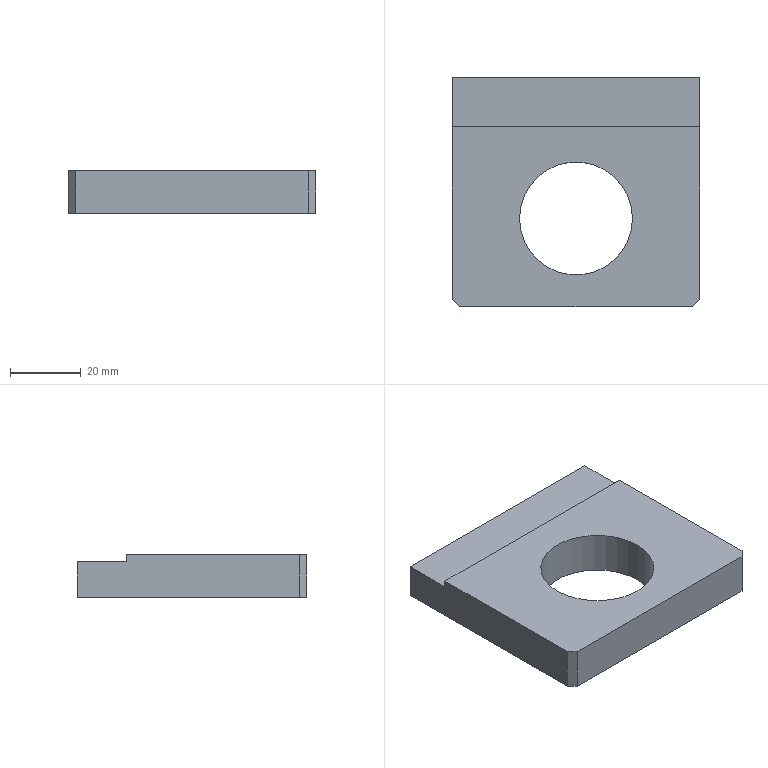Part | STEP file | Backup 2012-3-22-012 | 1 solid | 12 faces | box 70 x 65 x 12 mm | volume 42941 mm3 | plane 10 | cylinder 2 | commonest cylinder face diameters 32 x2
STEP:
#1=CARTESIAN_POINT('',(0.,0.,0.));
#2=DIRECTION('',(0.,0.,1.));
#3=DIRECTION('',(1.,0.,0.));
#4=AXIS2_PLACEMENT_3D('',#1,#2,#3);
#5=CARTESIAN_POINT('',(-16.,-7.5,12.));
#6=VERTEX_POINT('',#5);
#7=CARTESIAN_POINT('',(-16.,-7.5,0.));
#8=VERTEX_POINT('',#7);
#9=CARTESIAN_POINT('',(-16.,-7.5,12.));
#10=DIRECTION('',(0.,0.,-1.));
#11=VECTOR('',#10,1.);
#12=LINE('',#9,#11);
#13=CARTESIAN_POINT('',(0.,-7.5,12.));
#14=DIRECTION('',(0.,0.,-1.));
#15=DIRECTION('',(-1.,0.,0.));
#16=AXIS2_PLACEMENT_3D('',#13,#14,#15);
#17=CYLINDRICAL_SURFACE('',#16,16.);
#18=CARTESIAN_POINT('',(6.283,0.));
#19=DIRECTION('',(0.,1.));
#20=VECTOR('',#19,1.);
#21=LINE('',#18,#20);
#22=(GEOMETRIC_REPRESENTATION_CONTEXT(2)PARAMETRIC_REPRESENTATION_CONTEXT()REPRESENTATION_CONTEXT('',''));
#23=DEFINITIONAL_REPRESENTATION('',(#21),#22);
#24=PCURVE('',#17,#23);
#25=CARTESIAN_POINT('',(0.,-7.5,12.));
#26=DIRECTION('',(0.,0.,-1.));
#27=DIRECTION('',(-1.,0.,0.));
#28=AXIS2_PLACEMENT_3D('',#25,#26,#27);
#29=CYLINDRICAL_SURFACE('',#28,16.);
#30=CARTESIAN_POINT('',(0.,0.));
#31=DIRECTION('',(0.,1.));
#32=VECTOR('',#31,1.);
#33=LINE('',#30,#32);
#34=(GEOMETRIC_REPRESENTATION_CONTEXT(2)PARAMETRIC_REPRESENTATION_CONTEXT()REPRESENTATION_CONTEXT('',''));
#35=DEFINITIONAL_REPRESENTATION('',(#33),#34);
#36=PCURVE('',#29,#35);
#37=SURFACE_CURVE('',#12,(#24,#36),.PCURVE_S1.);
#38=EDGE_CURVE('',#6,#8,#37,.T.);
#39=ORIENTED_EDGE('',*,*,#38,.T.);
#40=CARTESIAN_POINT('',(16.,-7.5,0.));
#41=VERTEX_POINT('',#40);
#42=CARTESIAN_POINT('',(0.,-7.5,0.));
#43=DIRECTION('',(0.,0.,1.));
#44=DIRECTION('',(1.,0.,0.));
#45=AXIS2_PLACEMENT_3D('',#42,#43,#44);
#46=CIRCLE('',#45,16.);
#47=CARTESIAN_POINT('',(9.425,12.));
#48=DIRECTION('',(-1.,0.));
#49=VECTOR('',#48,1.);
#50=LINE('',#47,#49);
#51=(GEOMETRIC_REPRESENTATION_CONTEXT(2)PARAMETRIC_REPRESENTATION_CONTEXT()REPRESENTATION_CONTEXT('',''));
#52=DEFINITIONAL_REPRESENTATION('',(#50),#51);
#53=PCURVE('',#17,#52);
#54=CARTESIAN_POINT('',(35.,-32.5,0.));
#55=DIRECTION('',(0.,0.,1.));
#56=DIRECTION('',(1.,0.,0.));
#57=AXIS2_PLACEMENT_3D('',#54,#55,#56);
#58=PLANE('',#57);
#59=CARTESIAN_POINT('',(-35.,25.));
#60=DIRECTION('',(1.,0.));
#61=AXIS2_PLACEMENT_2D('',#59,#60);
#62=CIRCLE('',#61,16.);
#63=(GEOMETRIC_REPRESENTATION_CONTEXT(2)PARAMETRIC_REPRESENTATION_CONTEXT()REPRESENTATION_CONTEXT('',''));
#64=DEFINITIONAL_REPRESENTATION('',(#62),#63);
#65=PCURVE('',#58,#64);
#66=SURFACE_CURVE('',#46,(#53,#65),.PCURVE_S1.);
#67=EDGE_CURVE('',#8,#41,#66,.T.);
#68=ORIENTED_EDGE('',*,*,#67,.T.);
#69=CARTESIAN_POINT('',(16.,-7.5,12.));
#70=VERTEX_POINT('',#69);
#71=CARTESIAN_POINT('',(16.,-7.5,12.));
#72=DIRECTION('',(0.,0.,-1.));
#73=VECTOR('',#72,1.);
#74=LINE('',#71,#73);
#75=CARTESIAN_POINT('',(3.142,0.));
#76=DIRECTION('',(0.,1.));
#77=VECTOR('',#76,1.);
#78=LINE('',#75,#77);
#79=(GEOMETRIC_REPRESENTATION_CONTEXT(2)PARAMETRIC_REPRESENTATION_CONTEXT()REPRESENTATION_CONTEXT('',''));
#80=DEFINITIONAL_REPRESENTATION('',(#78),#79);
#81=PCURVE('',#17,#80);
#82=CARTESIAN_POINT('',(3.142,0.));
#83=DIRECTION('',(0.,1.));
#84=VECTOR('',#83,1.);
#85=LINE('',#82,#84);
#86=(GEOMETRIC_REPRESENTATION_CONTEXT(2)PARAMETRIC_REPRESENTATION_CONTEXT()REPRESENTATION_CONTEXT('',''));
#87=DEFINITIONAL_REPRESENTATION('',(#85),#86);
#88=PCURVE('',#29,#87);
#89=SURFACE_CURVE('',#74,(#81,#88),.PCURVE_S1.);
#90=EDGE_CURVE('',#70,#41,#89,.T.);
#91=ORIENTED_EDGE('',*,*,#90,.F.);
#92=CARTESIAN_POINT('',(0.,-7.5,12.));
#93=DIRECTION('',(0.,0.,1.));
#94=DIRECTION('',(1.,0.,0.));
#95=AXIS2_PLACEMENT_3D('',#92,#93,#94);
#96=CIRCLE('',#95,16.);
#97=CARTESIAN_POINT('',(9.425,0.));
#98=DIRECTION('',(-1.,0.));
#99=VECTOR('',#98,1.);
#100=LINE('',#97,#99);
#101=(GEOMETRIC_REPRESENTATION_CONTEXT(2)PARAMETRIC_REPRESENTATION_CONTEXT()REPRESENTATION_CONTEXT('',''));
#102=DEFINITIONAL_REPRESENTATION('',(#100),#101);
#103=PCURVE('',#17,#102);
#104=CARTESIAN_POINT('',(35.,-32.5,12.));
#105=DIRECTION('',(0.,0.,1.));
#106=DIRECTION('',(1.,0.,0.));
#107=AXIS2_PLACEMENT_3D('',#104,#105,#106);
#108=PLANE('',#107);
#109=CARTESIAN_POINT('',(-35.,25.));
#110=DIRECTION('',(1.,0.));
#111=AXIS2_PLACEMENT_2D('',#109,#110);
#112=CIRCLE('',#111,16.);
#113=(GEOMETRIC_REPRESENTATION_CONTEXT(2)PARAMETRIC_REPRESENTATION_CONTEXT()REPRESENTATION_CONTEXT('',''));
#114=DEFINITIONAL_REPRESENTATION('',(#112),#113);
#115=PCURVE('',#108,#114);
#116=SURFACE_CURVE('',#96,(#103,#115),.PCURVE_S1.);
#117=EDGE_CURVE('',#6,#70,#116,.T.);
#118=ORIENTED_EDGE('',*,*,#117,.F.);
#119=EDGE_LOOP('',(#39,#68,#91,#118));
#120=FACE_BOUND('',#119,.F.);
#121=ADVANCED_FACE('',(#120),#17,.F.);
#122=CARTESIAN_POINT('',(35.,32.5,10.));
#123=VERTEX_POINT('',#122);
#124=CARTESIAN_POINT('',(-35.,32.5,10.));
#125=VERTEX_POINT('',#124);
#126=CARTESIAN_POINT('',(-35.,32.5,10.));
#127=DIRECTION('',(-1.,0.,0.));
#128=VECTOR('',#127,1.);
#129=LINE('',#126,#128);
#130=CARTESIAN_POINT('',(-35.,32.5,12.));
#131=DIRECTION('',(0.,-1.,0.));
#132=DIRECTION('',(0.,0.,-1.));
#133=AXIS2_PLACEMENT_3D('',#130,#131,#132);
#134=PLANE('',#133);
#135=CARTESIAN_POINT('',(2.,0.));
#136=DIRECTION('',(0.,-1.));
#137=VECTOR('',#136,1.);
#138=LINE('',#135,#137);
#139=(GEOMETRIC_REPRESENTATION_CONTEXT(2)PARAMETRIC_REPRESENTATION_CONTEXT()REPRESENTATION_CONTEXT('',''));
#140=DEFINITIONAL_REPRESENTATION('',(#138),#139);
#141=PCURVE('',#134,#140);
#142=CARTESIAN_POINT('',(-35.,18.5,10.));
#143=DIRECTION('',(0.,0.,1.));
#144=DIRECTION('',(1.,0.,0.));
#145=AXIS2_PLACEMENT_3D('',#142,#143,#144);
#146=PLANE('',#145);
#147=CARTESIAN_POINT('',(0.,14.));
#148=DIRECTION('',(-1.,0.));
#149=VECTOR('',#148,1.);
#150=LINE('',#147,#149);
#151=(GEOMETRIC_REPRESENTATION_CONTEXT(2)PARAMETRIC_REPRESENTATION_CONTEXT()REPRESENTATION_CONTEXT('',''));
#152=DEFINITIONAL_REPRESENTATION('',(#150),#151);
#153=PCURVE('',#146,#152);
#154=SURFACE_CURVE('',#129,(#141,#153),.PCURVE_S1.);
#155=EDGE_CURVE('',#123,#125,#154,.T.);
#156=ORIENTED_EDGE('',*,*,#155,.F.);
#157=CARTESIAN_POINT('',(35.,32.5,0.));
#158=VERTEX_POINT('',#157);
#159=CARTESIAN_POINT('',(35.,32.5,12.));
#160=DIRECTION('',(0.,0.,-1.));
#161=VECTOR('',#160,1.);
#162=LINE('',#159,#161);
#163=CARTESIAN_POINT('',(0.,70.));
#164=DIRECTION('',(1.,0.));
#165=VECTOR('',#164,1.);
#166=LINE('',#163,#165);
#167=(GEOMETRIC_REPRESENTATION_CONTEXT(2)PARAMETRIC_REPRESENTATION_CONTEXT()REPRESENTATION_CONTEXT('',''));
#168=DEFINITIONAL_REPRESENTATION('',(#166),#167);
#169=PCURVE('',#134,#168);
#170=CARTESIAN_POINT('',(35.,32.5,12.));
#171=DIRECTION('',(-1.,0.,0.));
#172=DIRECTION('',(0.,-1.,0.));
#173=AXIS2_PLACEMENT_3D('',#170,#171,#172);
#174=PLANE('',#173);
#175=CARTESIAN_POINT('',(0.,0.));
#176=DIRECTION('',(0.,-1.));
#177=VECTOR('',#176,1.);
#178=LINE('',#175,#177);
#179=(GEOMETRIC_REPRESENTATION_CONTEXT(2)PARAMETRIC_REPRESENTATION_CONTEXT()REPRESENTATION_CONTEXT('',''));
#180=DEFINITIONAL_REPRESENTATION('',(#178),#179);
#181=PCURVE('',#174,#180);
#182=SURFACE_CURVE('',#162,(#169,#181),.PCURVE_S1.);
#183=EDGE_CURVE('',#123,#158,#182,.T.);
#184=ORIENTED_EDGE('',*,*,#183,.T.);
#185=CARTESIAN_POINT('',(-35.,32.5,0.));
#186=VERTEX_POINT('',#185);
#187=CARTESIAN_POINT('',(-35.,32.5,0.));
#188=DIRECTION('',(-1.,0.,0.));
#189=VECTOR('',#188,1.);
#190=LINE('',#187,#189);
#191=CARTESIAN_POINT('',(12.,0.));
#192=DIRECTION('',(0.,-1.));
#193=VECTOR('',#192,1.);
#194=LINE('',#191,#193);
#195=(GEOMETRIC_REPRESENTATION_CONTEXT(2)PARAMETRIC_REPRESENTATION_CONTEXT()REPRESENTATION_CONTEXT('',''));
#196=DEFINITIONAL_REPRESENTATION('',(#194),#195);
#197=PCURVE('',#134,#196);
#198=CARTESIAN_POINT('',(-70.,65.));
#199=DIRECTION('',(-1.,0.));
#200=VECTOR('',#199,1.);
#201=LINE('',#198,#200);
#202=(GEOMETRIC_REPRESENTATION_CONTEXT(2)PARAMETRIC_REPRESENTATION_CONTEXT()REPRESENTATION_CONTEXT('',''));
#203=DEFINITIONAL_REPRESENTATION('',(#201),#202);
#204=PCURVE('',#58,#203);
#205=SURFACE_CURVE('',#190,(#197,#204),.PCURVE_S1.);
#206=EDGE_CURVE('',#158,#186,#205,.T.);
#207=ORIENTED_EDGE('',*,*,#206,.T.);
#208=CARTESIAN_POINT('',(-35.,32.5,12.));
#209=DIRECTION('',(0.,0.,-1.));
#210=VECTOR('',#209,1.);
#211=LINE('',#208,#210);
#212=CARTESIAN_POINT('',(0.,0.));
#213=DIRECTION('',(1.,0.));
#214=VECTOR('',#213,1.);
#215=LINE('',#212,#214);
#216=(GEOMETRIC_REPRESENTATION_CONTEXT(2)PARAMETRIC_REPRESENTATION_CONTEXT()REPRESENTATION_CONTEXT('',''));
#217=DEFINITIONAL_REPRESENTATION('',(#215),#216);
#218=PCURVE('',#134,#217);
#219=CARTESIAN_POINT('',(-35.,32.5,12.));
#220=DIRECTION('',(1.,0.,0.));
#221=DIRECTION('',(0.,1.,0.));
#222=AXIS2_PLACEMENT_3D('',#219,#220,#221);
#223=PLANE('',#222);
#224=CARTESIAN_POINT('',(0.,0.));
#225=DIRECTION('',(0.,-1.));
#226=VECTOR('',#225,1.);
#227=LINE('',#224,#226);
#228=(GEOMETRIC_REPRESENTATION_CONTEXT(2)PARAMETRIC_REPRESENTATION_CONTEXT()REPRESENTATION_CONTEXT('',''));
#229=DEFINITIONAL_REPRESENTATION('',(#227),#228);
#230=PCURVE('',#223,#229);
#231=SURFACE_CURVE('',#211,(#218,#230),.PCURVE_S1.);
#232=EDGE_CURVE('',#125,#186,#231,.T.);
#233=ORIENTED_EDGE('',*,*,#232,.F.);
#234=EDGE_LOOP('',(#156,#184,#207,#233));
#235=FACE_BOUND('',#234,.T.);
#236=ADVANCED_FACE('',(#235),#134,.F.);
#237=CARTESIAN_POINT('',(-33.,-32.5,12.));
#238=VERTEX_POINT('',#237);
#239=CARTESIAN_POINT('',(33.,-32.5,12.));
#240=VERTEX_POINT('',#239);
#241=CARTESIAN_POINT('',(-35.,-32.5,12.));
#242=DIRECTION('',(1.,0.,0.));
#243=VECTOR('',#242,1.);
#244=LINE('',#241,#243);
#245=CARTESIAN_POINT('',(-70.,0.));
#246=DIRECTION('',(1.,0.));
#247=VECTOR('',#246,1.);
#248=LINE('',#245,#247);
#249=(GEOMETRIC_REPRESENTATION_CONTEXT(2)PARAMETRIC_REPRESENTATION_CONTEXT()REPRESENTATION_CONTEXT('',''));
#250=DEFINITIONAL_REPRESENTATION('',(#248),#249);
#251=PCURVE('',#108,#250);
#252=CARTESIAN_POINT('',(-35.,-32.5,12.));
#253=DIRECTION('',(0.,1.,0.));
#254=DIRECTION('',(0.,0.,1.));
#255=AXIS2_PLACEMENT_3D('',#252,#253,#254);
#256=PLANE('',#255);
#257=CARTESIAN_POINT('',(0.,0.));
#258=DIRECTION('',(0.,1.));
#259=VECTOR('',#258,1.);
#260=LINE('',#257,#259);
#261=(GEOMETRIC_REPRESENTATION_CONTEXT(2)PARAMETRIC_REPRESENTATION_CONTEXT()REPRESENTATION_CONTEXT('',''));
#262=DEFINITIONAL_REPRESENTATION('',(#260),#261);
#263=PCURVE('',#256,#262);
#264=SURFACE_CURVE('',#244,(#251,#263),.PCURVE_S1.);
#265=EDGE_CURVE('',#238,#240,#264,.T.);
#266=ORIENTED_EDGE('',*,*,#265,.T.);
#267=CARTESIAN_POINT('',(35.,-30.5,12.));
#268=VERTEX_POINT('',#267);
#269=CARTESIAN_POINT('',(34.,-31.5,12.));
#270=DIRECTION('',(0.7071,0.7071,0.));
#271=VECTOR('',#270,1.);
#272=LINE('',#269,#271);
#273=CARTESIAN_POINT('',(-1.,1.));
#274=DIRECTION('',(0.7071,0.7071));
#275=VECTOR('',#274,1.);
#276=LINE('',#273,#275);
#277=(GEOMETRIC_REPRESENTATION_CONTEXT(2)PARAMETRIC_REPRESENTATION_CONTEXT()REPRESENTATION_CONTEXT('',''));
#278=DEFINITIONAL_REPRESENTATION('',(#276),#277);
#279=PCURVE('',#108,#278);
#280=CARTESIAN_POINT('',(35.,-30.5,12.));
#281=DIRECTION('',(-0.7071,0.7071,0.));
#282=DIRECTION('',(-0.7071,-0.7071,0.));
#283=AXIS2_PLACEMENT_3D('',#280,#281,#282);
#284=PLANE('',#283);
#285=CARTESIAN_POINT('',(1.414,0.));
#286=DIRECTION('',(-1.,0.));
#287=VECTOR('',#286,1.);
#288=LINE('',#285,#287);
#289=(GEOMETRIC_REPRESENTATION_CONTEXT(2)PARAMETRIC_REPRESENTATION_CONTEXT()REPRESENTATION_CONTEXT('',''));
#290=DEFINITIONAL_REPRESENTATION('',(#288),#289);
#291=PCURVE('',#284,#290);
#292=SURFACE_CURVE('',#272,(#279,#291),.PCURVE_S1.);
#293=EDGE_CURVE('',#240,#268,#292,.T.);
#294=ORIENTED_EDGE('',*,*,#293,.T.);
#295=CARTESIAN_POINT('',(35.,18.5,12.));
#296=VERTEX_POINT('',#295);
#297=CARTESIAN_POINT('',(35.,32.5,12.));
#298=DIRECTION('',(0.,1.,0.));
#299=VECTOR('',#298,1.);
#300=LINE('',#297,#299);
#301=CARTESIAN_POINT('',(0.,65.));
#302=DIRECTION('',(0.,1.));
#303=VECTOR('',#302,1.);
#304=LINE('',#301,#303);
#305=(GEOMETRIC_REPRESENTATION_CONTEXT(2)PARAMETRIC_REPRESENTATION_CONTEXT()REPRESENTATION_CONTEXT('',''));
#306=DEFINITIONAL_REPRESENTATION('',(#304),#305);
#307=PCURVE('',#108,#306);
#308=CARTESIAN_POINT('',(0.,0.));
#309=DIRECTION('',(-1.,0.));
#310=VECTOR('',#309,1.);
#311=LINE('',#308,#310);
#312=(GEOMETRIC_REPRESENTATION_CONTEXT(2)PARAMETRIC_REPRESENTATION_CONTEXT()REPRESENTATION_CONTEXT('',''));
#313=DEFINITIONAL_REPRESENTATION('',(#311),#312);
#314=PCURVE('',#174,#313);
#315=SURFACE_CURVE('',#300,(#307,#314),.PCURVE_S1.);
#316=EDGE_CURVE('',#268,#296,#315,.T.);
#317=ORIENTED_EDGE('',*,*,#316,.T.);
#318=CARTESIAN_POINT('',(-35.,18.5,12.));
#319=VERTEX_POINT('',#318);
#320=CARTESIAN_POINT('',(-35.,18.5,12.));
#321=DIRECTION('',(1.,0.,0.));
#322=VECTOR('',#321,1.);
#323=LINE('',#320,#322);
#324=CARTESIAN_POINT('',(-70.,51.));
#325=DIRECTION('',(1.,0.));
#326=VECTOR('',#325,1.);
#327=LINE('',#324,#326);
#328=(GEOMETRIC_REPRESENTATION_CONTEXT(2)PARAMETRIC_REPRESENTATION_CONTEXT()REPRESENTATION_CONTEXT('',''));
#329=DEFINITIONAL_REPRESENTATION('',(#327),#328);
#330=PCURVE('',#108,#329);
#331=CARTESIAN_POINT('',(-35.,18.5,10.));
#332=DIRECTION('',(0.,-1.,0.));
#333=DIRECTION('',(1.,0.,0.));
#334=AXIS2_PLACEMENT_3D('',#331,#332,#333);
#335=PLANE('',#334);
#336=CARTESIAN_POINT('',(0.,2.));
#337=DIRECTION('',(1.,0.));
#338=VECTOR('',#337,1.);
#339=LINE('',#336,#338);
#340=(GEOMETRIC_REPRESENTATION_CONTEXT(2)PARAMETRIC_REPRESENTATION_CONTEXT()REPRESENTATION_CONTEXT('',''));
#341=DEFINITIONAL_REPRESENTATION('',(#339),#340);
#342=PCURVE('',#335,#341);
#343=SURFACE_CURVE('',#323,(#330,#342),.PCURVE_S1.);
#344=EDGE_CURVE('',#319,#296,#343,.T.);
#345=ORIENTED_EDGE('',*,*,#344,.F.);
#346=CARTESIAN_POINT('',(-35.,-30.5,12.));
#347=VERTEX_POINT('',#346);
#348=CARTESIAN_POINT('',(-35.,32.5,12.));
#349=DIRECTION('',(0.,-1.,0.));
#350=VECTOR('',#349,1.);
#351=LINE('',#348,#350);
#352=CARTESIAN_POINT('',(-70.,65.));
#353=DIRECTION('',(0.,-1.));
#354=VECTOR('',#353,1.);
#355=LINE('',#352,#354);
#356=(GEOMETRIC_REPRESENTATION_CONTEXT(2)PARAMETRIC_REPRESENTATION_CONTEXT()REPRESENTATION_CONTEXT('',''));
#357=DEFINITIONAL_REPRESENTATION('',(#355),#356);
#358=PCURVE('',#108,#357);
#359=CARTESIAN_POINT('',(0.,0.));
#360=DIRECTION('',(-1.,0.));
#361=VECTOR('',#360,1.);
#362=LINE('',#359,#361);
#363=(GEOMETRIC_REPRESENTATION_CONTEXT(2)PARAMETRIC_REPRESENTATION_CONTEXT()REPRESENTATION_CONTEXT('',''));
#364=DEFINITIONAL_REPRESENTATION('',(#362),#363);
#365=PCURVE('',#223,#364);
#366=SURFACE_CURVE('',#351,(#358,#365),.PCURVE_S1.);
#367=EDGE_CURVE('',#319,#347,#366,.T.);
#368=ORIENTED_EDGE('',*,*,#367,.T.);
#369=CARTESIAN_POINT('',(1.,-66.5,12.));
#370=DIRECTION('',(0.7071,-0.7071,0.));
#371=VECTOR('',#370,1.);
#372=LINE('',#369,#371);
#373=CARTESIAN_POINT('',(-34.,-34.));
#374=DIRECTION('',(0.7071,-0.7071));
#375=VECTOR('',#374,1.);
#376=LINE('',#373,#375);
#377=(GEOMETRIC_REPRESENTATION_CONTEXT(2)PARAMETRIC_REPRESENTATION_CONTEXT()REPRESENTATION_CONTEXT('',''));
#378=DEFINITIONAL_REPRESENTATION('',(#376),#377);
#379=PCURVE('',#108,#378);
#380=CARTESIAN_POINT('',(-33.,-32.5,12.));
#381=DIRECTION('',(0.7071,0.7071,0.));
#382=DIRECTION('',(-0.7071,0.7071,0.));
#383=AXIS2_PLACEMENT_3D('',#380,#381,#382);
#384=PLANE('',#383);
#385=CARTESIAN_POINT('',(-48.083,0.));
#386=DIRECTION('',(-1.,0.));
#387=VECTOR('',#386,1.);
#388=LINE('',#385,#387);
#389=(GEOMETRIC_REPRESENTATION_CONTEXT(2)PARAMETRIC_REPRESENTATION_CONTEXT()REPRESENTATION_CONTEXT('',''));
#390=DEFINITIONAL_REPRESENTATION('',(#388),#389);
#391=PCURVE('',#384,#390);
#392=SURFACE_CURVE('',#372,(#379,#391),.PCURVE_S1.);
#393=EDGE_CURVE('',#347,#238,#392,.T.);
#394=ORIENTED_EDGE('',*,*,#393,.T.);
#395=EDGE_LOOP('',(#266,#294,#317,#345,#368,#394));
#396=FACE_BOUND('',#395,.T.);
#397=ORIENTED_EDGE('',*,*,#117,.F.);
#398=CARTESIAN_POINT('',(0.,-7.5,12.));
#399=DIRECTION('',(0.,0.,1.));
#400=DIRECTION('',(1.,0.,0.));
#401=AXIS2_PLACEMENT_3D('',#398,#399,#400);
#402=CIRCLE('',#401,16.);
#403=CARTESIAN_POINT('',(-35.,25.));
#404=DIRECTION('',(1.,0.));
#405=AXIS2_PLACEMENT_2D('',#403,#404);
#406=CIRCLE('',#405,16.);
#407=(GEOMETRIC_REPRESENTATION_CONTEXT(2)PARAMETRIC_REPRESENTATION_CONTEXT()REPRESENTATION_CONTEXT('',''));
#408=DEFINITIONAL_REPRESENTATION('',(#406),#407);
#409=PCURVE('',#108,#408);
#410=CARTESIAN_POINT('',(3.142,0.));
#411=DIRECTION('',(-1.,0.));
#412=VECTOR('',#411,1.);
#413=LINE('',#410,#412);
#414=(GEOMETRIC_REPRESENTATION_CONTEXT(2)PARAMETRIC_REPRESENTATION_CONTEXT()REPRESENTATION_CONTEXT('',''));
#415=DEFINITIONAL_REPRESENTATION('',(#413),#414);
#416=PCURVE('',#29,#415);
#417=SURFACE_CURVE('',#402,(#409,#416),.PCURVE_S1.);
#418=EDGE_CURVE('',#70,#6,#417,.T.);
#419=ORIENTED_EDGE('',*,*,#418,.F.);
#420=EDGE_LOOP('',(#397,#419));
#421=FACE_BOUND('',#420,.T.);
#422=ADVANCED_FACE('',(#396,#421),#108,.T.);
#423=CARTESIAN_POINT('',(35.,-30.5,0.));
#424=VERTEX_POINT('',#423);
#425=CARTESIAN_POINT('',(35.,32.5,0.));
#426=DIRECTION('',(0.,1.,0.));
#427=VECTOR('',#426,1.);
#428=LINE('',#425,#427);
#429=CARTESIAN_POINT('',(0.,65.));
#430=DIRECTION('',(0.,1.));
#431=VECTOR('',#430,1.);
#432=LINE('',#429,#431);
#433=(GEOMETRIC_REPRESENTATION_CONTEXT(2)PARAMETRIC_REPRESENTATION_CONTEXT()REPRESENTATION_CONTEXT('',''));
#434=DEFINITIONAL_REPRESENTATION('',(#432),#433);
#435=PCURVE('',#58,#434);
#436=CARTESIAN_POINT('',(0.,-12.));
#437=DIRECTION('',(-1.,0.));
#438=VECTOR('',#437,1.);
#439=LINE('',#436,#438);
#440=(GEOMETRIC_REPRESENTATION_CONTEXT(2)PARAMETRIC_REPRESENTATION_CONTEXT()REPRESENTATION_CONTEXT('',''));
#441=DEFINITIONAL_REPRESENTATION('',(#439),#440);
#442=PCURVE('',#174,#441);
#443=SURFACE_CURVE('',#428,(#435,#442),.PCURVE_S1.);
#444=EDGE_CURVE('',#424,#158,#443,.T.);
#445=ORIENTED_EDGE('',*,*,#444,.F.);
#446=CARTESIAN_POINT('',(33.,-32.5,0.));
#447=VERTEX_POINT('',#446);
#448=CARTESIAN_POINT('',(35.,-30.5,0.));
#449=DIRECTION('',(-0.7071,-0.7071,0.));
#450=VECTOR('',#449,1.);
#451=LINE('',#448,#450);
#452=CARTESIAN_POINT('',(0.,2.));
#453=DIRECTION('',(-0.7071,-0.7071));
#454=VECTOR('',#453,1.);
#455=LINE('',#452,#454);
#456=(GEOMETRIC_REPRESENTATION_CONTEXT(2)PARAMETRIC_REPRESENTATION_CONTEXT()REPRESENTATION_CONTEXT('',''));
#457=DEFINITIONAL_REPRESENTATION('',(#455),#456);
#458=PCURVE('',#58,#457);
#459=CARTESIAN_POINT('',(0.,-12.));
#460=DIRECTION('',(1.,0.));
#461=VECTOR('',#460,1.);
#462=LINE('',#459,#461);
#463=(GEOMETRIC_REPRESENTATION_CONTEXT(2)PARAMETRIC_REPRESENTATION_CONTEXT()REPRESENTATION_CONTEXT('',''));
#464=DEFINITIONAL_REPRESENTATION('',(#462),#463);
#465=PCURVE('',#284,#464);
#466=SURFACE_CURVE('',#451,(#458,#465),.PCURVE_S1.);
#467=EDGE_CURVE('',#424,#447,#466,.T.);
#468=ORIENTED_EDGE('',*,*,#467,.T.);
#469=CARTESIAN_POINT('',(-33.,-32.5,0.));
#470=VERTEX_POINT('',#469);
#471=CARTESIAN_POINT('',(-35.,-32.5,0.));
#472=DIRECTION('',(1.,0.,0.));
#473=VECTOR('',#472,1.);
#474=LINE('',#471,#473);
#475=CARTESIAN_POINT('',(-70.,0.));
#476=DIRECTION('',(1.,0.));
#477=VECTOR('',#476,1.);
#478=LINE('',#475,#477);
#479=(GEOMETRIC_REPRESENTATION_CONTEXT(2)PARAMETRIC_REPRESENTATION_CONTEXT()REPRESENTATION_CONTEXT('',''));
#480=DEFINITIONAL_REPRESENTATION('',(#478),#479);
#481=PCURVE('',#58,#480);
#482=CARTESIAN_POINT('',(-12.,0.));
#483=DIRECTION('',(0.,1.));
#484=VECTOR('',#483,1.);
#485=LINE('',#482,#484);
#486=(GEOMETRIC_REPRESENTATION_CONTEXT(2)PARAMETRIC_REPRESENTATION_CONTEXT()REPRESENTATION_CONTEXT('',''));
#487=DEFINITIONAL_REPRESENTATION('',(#485),#486);
#488=PCURVE('',#256,#487);
#489=SURFACE_CURVE('',#474,(#481,#488),.PCURVE_S1.);
#490=EDGE_CURVE('',#470,#447,#489,.T.);
#491=ORIENTED_EDGE('',*,*,#490,.F.);
#492=CARTESIAN_POINT('',(-35.,-30.5,0.));
#493=VERTEX_POINT('',#492);
#494=CARTESIAN_POINT('',(-33.,-32.5,0.));
#495=DIRECTION('',(-0.7071,0.7071,0.));
#496=VECTOR('',#495,1.);
#497=LINE('',#494,#496);
#498=CARTESIAN_POINT('',(-68.,0.));
#499=DIRECTION('',(-0.7071,0.7071));
#500=VECTOR('',#499,1.);
#501=LINE('',#498,#500);
#502=(GEOMETRIC_REPRESENTATION_CONTEXT(2)PARAMETRIC_REPRESENTATION_CONTEXT()REPRESENTATION_CONTEXT('',''));
#503=DEFINITIONAL_REPRESENTATION('',(#501),#502);
#504=PCURVE('',#58,#503);
#505=CARTESIAN_POINT('',(0.,-12.));
#506=DIRECTION('',(1.,0.));
#507=VECTOR('',#506,1.);
#508=LINE('',#505,#507);
#509=(GEOMETRIC_REPRESENTATION_CONTEXT(2)PARAMETRIC_REPRESENTATION_CONTEXT()REPRESENTATION_CONTEXT('',''));
#510=DEFINITIONAL_REPRESENTATION('',(#508),#509);
#511=PCURVE('',#384,#510);
#512=SURFACE_CURVE('',#497,(#504,#511),.PCURVE_S1.);
#513=EDGE_CURVE('',#470,#493,#512,.T.);
#514=ORIENTED_EDGE('',*,*,#513,.T.);
#515=CARTESIAN_POINT('',(-35.,32.5,0.));
#516=DIRECTION('',(0.,-1.,0.));
#517=VECTOR('',#516,1.);
#518=LINE('',#515,#517);
#519=CARTESIAN_POINT('',(-70.,65.));
#520=DIRECTION('',(0.,-1.));
#521=VECTOR('',#520,1.);
#522=LINE('',#519,#521);
#523=(GEOMETRIC_REPRESENTATION_CONTEXT(2)PARAMETRIC_REPRESENTATION_CONTEXT()REPRESENTATION_CONTEXT('',''));
#524=DEFINITIONAL_REPRESENTATION('',(#522),#523);
#525=PCURVE('',#58,#524);
#526=CARTESIAN_POINT('',(0.,-12.));
#527=DIRECTION('',(-1.,0.));
#528=VECTOR('',#527,1.);
#529=LINE('',#526,#528);
#530=(GEOMETRIC_REPRESENTATION_CONTEXT(2)PARAMETRIC_REPRESENTATION_CONTEXT()REPRESENTATION_CONTEXT('',''));
#531=DEFINITIONAL_REPRESENTATION('',(#529),#530);
#532=PCURVE('',#223,#531);
#533=SURFACE_CURVE('',#518,(#525,#532),.PCURVE_S1.);
#534=EDGE_CURVE('',#186,#493,#533,.T.);
#535=ORIENTED_EDGE('',*,*,#534,.F.);
#536=ORIENTED_EDGE('',*,*,#206,.F.);
#537=EDGE_LOOP('',(#445,#468,#491,#514,#535,#536));
#538=FACE_BOUND('',#537,.T.);
#539=ORIENTED_EDGE('',*,*,#67,.T.);
#540=CARTESIAN_POINT('',(0.,-7.5,0.));
#541=DIRECTION('',(0.,0.,1.));
#542=DIRECTION('',(1.,0.,0.));
#543=AXIS2_PLACEMENT_3D('',#540,#541,#542);
#544=CIRCLE('',#543,16.);
#545=CARTESIAN_POINT('',(-35.,25.));
#546=DIRECTION('',(1.,0.));
#547=AXIS2_PLACEMENT_2D('',#545,#546);
#548=CIRCLE('',#547,16.);
#549=(GEOMETRIC_REPRESENTATION_CONTEXT(2)PARAMETRIC_REPRESENTATION_CONTEXT()REPRESENTATION_CONTEXT('',''));
#550=DEFINITIONAL_REPRESENTATION('',(#548),#549);
#551=PCURVE('',#58,#550);
#552=CARTESIAN_POINT('',(3.142,12.));
#553=DIRECTION('',(-1.,0.));
#554=VECTOR('',#553,1.);
#555=LINE('',#552,#554);
#556=(GEOMETRIC_REPRESENTATION_CONTEXT(2)PARAMETRIC_REPRESENTATION_CONTEXT()REPRESENTATION_CONTEXT('',''));
#557=DEFINITIONAL_REPRESENTATION('',(#555),#556);
#558=PCURVE('',#29,#557);
#559=SURFACE_CURVE('',#544,(#551,#558),.PCURVE_S1.);
#560=EDGE_CURVE('',#41,#8,#559,.T.);
#561=ORIENTED_EDGE('',*,*,#560,.T.);
#562=EDGE_LOOP('',(#539,#561));
#563=FACE_BOUND('',#562,.T.);
#564=ADVANCED_FACE('',(#538,#563),#58,.F.);
#565=ORIENTED_EDGE('',*,*,#316,.F.);
#566=CARTESIAN_POINT('',(35.,-30.5,12.));
#567=DIRECTION('',(0.,0.,-1.));
#568=VECTOR('',#567,1.);
#569=LINE('',#566,#568);
#570=CARTESIAN_POINT('',(63.,0.));
#571=DIRECTION('',(0.,-1.));
#572=VECTOR('',#571,1.);
#573=LINE('',#570,#572);
#574=(GEOMETRIC_REPRESENTATION_CONTEXT(2)PARAMETRIC_REPRESENTATION_CONTEXT()REPRESENTATION_CONTEXT('',''));
#575=DEFINITIONAL_REPRESENTATION('',(#573),#574);
#576=PCURVE('',#174,#575);
#577=CARTESIAN_POINT('',(0.,0.));
#578=DIRECTION('',(0.,-1.));
#579=VECTOR('',#578,1.);
#580=LINE('',#577,#579);
#581=(GEOMETRIC_REPRESENTATION_CONTEXT(2)PARAMETRIC_REPRESENTATION_CONTEXT()REPRESENTATION_CONTEXT('',''));
#582=DEFINITIONAL_REPRESENTATION('',(#580),#581);
#583=PCURVE('',#284,#582);
#584=SURFACE_CURVE('',#569,(#576,#583),.PCURVE_S1.);
#585=EDGE_CURVE('',#268,#424,#584,.T.);
#586=ORIENTED_EDGE('',*,*,#585,.T.);
#587=ORIENTED_EDGE('',*,*,#444,.T.);
#588=ORIENTED_EDGE('',*,*,#183,.F.);
#589=CARTESIAN_POINT('',(35.,18.5,10.));
#590=VERTEX_POINT('',#589);
#591=CARTESIAN_POINT('',(35.,32.5,10.));
#592=DIRECTION('',(0.,1.,0.));
#593=VECTOR('',#592,1.);
#594=LINE('',#591,#593);
#595=CARTESIAN_POINT('',(0.,-2.));
#596=DIRECTION('',(-1.,0.));
#597=VECTOR('',#596,1.);
#598=LINE('',#595,#597);
#599=(GEOMETRIC_REPRESENTATION_CONTEXT(2)PARAMETRIC_REPRESENTATION_CONTEXT()REPRESENTATION_CONTEXT('',''));
#600=DEFINITIONAL_REPRESENTATION('',(#598),#599);
#601=PCURVE('',#174,#600);
#602=CARTESIAN_POINT('',(70.,14.));
#603=DIRECTION('',(0.,1.));
#604=VECTOR('',#603,1.);
#605=LINE('',#602,#604);
#606=(GEOMETRIC_REPRESENTATION_CONTEXT(2)PARAMETRIC_REPRESENTATION_CONTEXT()REPRESENTATION_CONTEXT('',''));
#607=DEFINITIONAL_REPRESENTATION('',(#605),#606);
#608=PCURVE('',#146,#607);
#609=SURFACE_CURVE('',#594,(#601,#608),.PCURVE_S1.);
#610=EDGE_CURVE('',#590,#123,#609,.T.);
#611=ORIENTED_EDGE('',*,*,#610,.F.);
#612=CARTESIAN_POINT('',(35.,18.5,10.));
#613=DIRECTION('',(0.,0.,1.));
#614=VECTOR('',#613,1.);
#615=LINE('',#612,#614);
#616=CARTESIAN_POINT('',(14.,-2.));
#617=DIRECTION('',(0.,1.));
#618=VECTOR('',#617,1.);
#619=LINE('',#616,#618);
#620=(GEOMETRIC_REPRESENTATION_CONTEXT(2)PARAMETRIC_REPRESENTATION_CONTEXT()REPRESENTATION_CONTEXT('',''));
#621=DEFINITIONAL_REPRESENTATION('',(#619),#620);
#622=PCURVE('',#174,#621);
#623=CARTESIAN_POINT('',(70.,0.));
#624=DIRECTION('',(0.,1.));
#625=VECTOR('',#624,1.);
#626=LINE('',#623,#625);
#627=(GEOMETRIC_REPRESENTATION_CONTEXT(2)PARAMETRIC_REPRESENTATION_CONTEXT()REPRESENTATION_CONTEXT('',''));
#628=DEFINITIONAL_REPRESENTATION('',(#626),#627);
#629=PCURVE('',#335,#628);
#630=SURFACE_CURVE('',#615,(#622,#629),.PCURVE_S1.);
#631=EDGE_CURVE('',#590,#296,#630,.T.);
#632=ORIENTED_EDGE('',*,*,#631,.T.);
#633=EDGE_LOOP('',(#565,#586,#587,#588,#611,#632));
#634=FACE_BOUND('',#633,.T.);
#635=ADVANCED_FACE('',(#634),#174,.F.);
#636=ORIENTED_EDGE('',*,*,#534,.T.);
#637=CARTESIAN_POINT('',(-35.,-30.5,12.));
#638=DIRECTION('',(0.,0.,1.));
#639=VECTOR('',#638,1.);
#640=LINE('',#637,#639);
#641=CARTESIAN_POINT('',(-63.,0.));
#642=DIRECTION('',(0.,1.));
#643=VECTOR('',#642,1.);
#644=LINE('',#641,#643);
#645=(GEOMETRIC_REPRESENTATION_CONTEXT(2)PARAMETRIC_REPRESENTATION_CONTEXT()REPRESENTATION_CONTEXT('',''));
#646=DEFINITIONAL_REPRESENTATION('',(#644),#645);
#647=PCURVE('',#223,#646);
#648=CARTESIAN_POINT('',(2.828,0.));
#649=DIRECTION('',(0.,1.));
#650=VECTOR('',#649,1.);
#651=LINE('',#648,#650);
#652=(GEOMETRIC_REPRESENTATION_CONTEXT(2)PARAMETRIC_REPRESENTATION_CONTEXT()REPRESENTATION_CONTEXT('',''));
#653=DEFINITIONAL_REPRESENTATION('',(#651),#652);
#654=PCURVE('',#384,#653);
#655=SURFACE_CURVE('',#640,(#647,#654),.PCURVE_S1.);
#656=EDGE_CURVE('',#493,#347,#655,.T.);
#657=ORIENTED_EDGE('',*,*,#656,.T.);
#658=ORIENTED_EDGE('',*,*,#367,.F.);
#659=CARTESIAN_POINT('',(-35.,18.5,10.));
#660=VERTEX_POINT('',#659);
#661=CARTESIAN_POINT('',(-35.,18.5,10.));
#662=DIRECTION('',(0.,0.,1.));
#663=VECTOR('',#662,1.);
#664=LINE('',#661,#663);
#665=CARTESIAN_POINT('',(-14.,-2.));
#666=DIRECTION('',(0.,1.));
#667=VECTOR('',#666,1.);
#668=LINE('',#665,#667);
#669=(GEOMETRIC_REPRESENTATION_CONTEXT(2)PARAMETRIC_REPRESENTATION_CONTEXT()REPRESENTATION_CONTEXT('',''));
#670=DEFINITIONAL_REPRESENTATION('',(#668),#669);
#671=PCURVE('',#223,#670);
#672=CARTESIAN_POINT('',(0.,0.));
#673=DIRECTION('',(0.,1.));
#674=VECTOR('',#673,1.);
#675=LINE('',#672,#674);
#676=(GEOMETRIC_REPRESENTATION_CONTEXT(2)PARAMETRIC_REPRESENTATION_CONTEXT()REPRESENTATION_CONTEXT('',''));
#677=DEFINITIONAL_REPRESENTATION('',(#675),#676);
#678=PCURVE('',#335,#677);
#679=SURFACE_CURVE('',#664,(#671,#678),.PCURVE_S1.);
#680=EDGE_CURVE('',#660,#319,#679,.T.);
#681=ORIENTED_EDGE('',*,*,#680,.F.);
#682=CARTESIAN_POINT('',(-35.,32.5,10.));
#683=DIRECTION('',(0.,-1.,0.));
#684=VECTOR('',#683,1.);
#685=LINE('',#682,#684);
#686=CARTESIAN_POINT('',(0.,-2.));
#687=DIRECTION('',(-1.,0.));
#688=VECTOR('',#687,1.);
#689=LINE('',#686,#688);
#690=(GEOMETRIC_REPRESENTATION_CONTEXT(2)PARAMETRIC_REPRESENTATION_CONTEXT()REPRESENTATION_CONTEXT('',''));
#691=DEFINITIONAL_REPRESENTATION('',(#689),#690);
#692=PCURVE('',#223,#691);
#693=CARTESIAN_POINT('',(0.,14.));
#694=DIRECTION('',(0.,-1.));
#695=VECTOR('',#694,1.);
#696=LINE('',#693,#695);
#697=(GEOMETRIC_REPRESENTATION_CONTEXT(2)PARAMETRIC_REPRESENTATION_CONTEXT()REPRESENTATION_CONTEXT('',''));
#698=DEFINITIONAL_REPRESENTATION('',(#696),#697);
#699=PCURVE('',#146,#698);
#700=SURFACE_CURVE('',#685,(#692,#699),.PCURVE_S1.);
#701=EDGE_CURVE('',#125,#660,#700,.T.);
#702=ORIENTED_EDGE('',*,*,#701,.F.);
#703=ORIENTED_EDGE('',*,*,#232,.T.);
#704=EDGE_LOOP('',(#636,#657,#658,#681,#702,#703));
#705=FACE_BOUND('',#704,.T.);
#706=ADVANCED_FACE('',(#705),#223,.F.);
#707=ORIENTED_EDGE('',*,*,#490,.T.);
#708=CARTESIAN_POINT('',(33.,-32.5,12.));
#709=DIRECTION('',(0.,0.,1.));
#710=VECTOR('',#709,1.);
#711=LINE('',#708,#710);
#712=CARTESIAN_POINT('',(0.,68.));
#713=DIRECTION('',(1.,0.));
#714=VECTOR('',#713,1.);
#715=LINE('',#712,#714);
#716=(GEOMETRIC_REPRESENTATION_CONTEXT(2)PARAMETRIC_REPRESENTATION_CONTEXT()REPRESENTATION_CONTEXT('',''));
#717=DEFINITIONAL_REPRESENTATION('',(#715),#716);
#718=PCURVE('',#256,#717);
#719=CARTESIAN_POINT('',(2.828,0.));
#720=DIRECTION('',(0.,1.));
#721=VECTOR('',#720,1.);
#722=LINE('',#719,#721);
#723=(GEOMETRIC_REPRESENTATION_CONTEXT(2)PARAMETRIC_REPRESENTATION_CONTEXT()REPRESENTATION_CONTEXT('',''));
#724=DEFINITIONAL_REPRESENTATION('',(#722),#723);
#725=PCURVE('',#284,#724);
#726=SURFACE_CURVE('',#711,(#718,#725),.PCURVE_S1.);
#727=EDGE_CURVE('',#447,#240,#726,.T.);
#728=ORIENTED_EDGE('',*,*,#727,.T.);
#729=ORIENTED_EDGE('',*,*,#265,.F.);
#730=CARTESIAN_POINT('',(-33.,-32.5,12.));
#731=DIRECTION('',(0.,0.,-1.));
#732=VECTOR('',#731,1.);
#733=LINE('',#730,#732);
#734=CARTESIAN_POINT('',(0.,2.));
#735=DIRECTION('',(-1.,0.));
#736=VECTOR('',#735,1.);
#737=LINE('',#734,#736);
#738=(GEOMETRIC_REPRESENTATION_CONTEXT(2)PARAMETRIC_REPRESENTATION_CONTEXT()REPRESENTATION_CONTEXT('',''));
#739=DEFINITIONAL_REPRESENTATION('',(#737),#738);
#740=PCURVE('',#256,#739);
#741=CARTESIAN_POINT('',(0.,0.));
#742=DIRECTION('',(0.,-1.));
#743=VECTOR('',#742,1.);
#744=LINE('',#741,#743);
#745=(GEOMETRIC_REPRESENTATION_CONTEXT(2)PARAMETRIC_REPRESENTATION_CONTEXT()REPRESENTATION_CONTEXT('',''));
#746=DEFINITIONAL_REPRESENTATION('',(#744),#745);
#747=PCURVE('',#384,#746);
#748=SURFACE_CURVE('',#733,(#740,#747),.PCURVE_S1.);
#749=EDGE_CURVE('',#238,#470,#748,.T.);
#750=ORIENTED_EDGE('',*,*,#749,.T.);
#751=EDGE_LOOP('',(#707,#728,#729,#750));
#752=FACE_BOUND('',#751,.T.);
#753=ADVANCED_FACE('',(#752),#256,.F.);
#754=ORIENTED_EDGE('',*,*,#560,.T.);
#755=ORIENTED_EDGE('',*,*,#38,.F.);
#756=ORIENTED_EDGE('',*,*,#418,.F.);
#757=ORIENTED_EDGE('',*,*,#90,.T.);
#758=EDGE_LOOP('',(#754,#755,#756,#757));
#759=FACE_BOUND('',#758,.F.);
#760=ADVANCED_FACE('',(#759),#29,.F.);
#761=ORIENTED_EDGE('',*,*,#344,.T.);
#762=ORIENTED_EDGE('',*,*,#631,.F.);
#763=CARTESIAN_POINT('',(-35.,18.5,10.));
#764=DIRECTION('',(1.,0.,0.));
#765=VECTOR('',#764,1.);
#766=LINE('',#763,#765);
#767=CARTESIAN_POINT('',(0.,0.));
#768=DIRECTION('',(1.,0.));
#769=VECTOR('',#768,1.);
#770=LINE('',#767,#769);
#771=(GEOMETRIC_REPRESENTATION_CONTEXT(2)PARAMETRIC_REPRESENTATION_CONTEXT()REPRESENTATION_CONTEXT('',''));
#772=DEFINITIONAL_REPRESENTATION('',(#770),#771);
#773=PCURVE('',#335,#772);
#774=CARTESIAN_POINT('',(0.,0.));
#775=DIRECTION('',(1.,0.));
#776=VECTOR('',#775,1.);
#777=LINE('',#774,#776);
#778=(GEOMETRIC_REPRESENTATION_CONTEXT(2)PARAMETRIC_REPRESENTATION_CONTEXT()REPRESENTATION_CONTEXT('',''));
#779=DEFINITIONAL_REPRESENTATION('',(#777),#778);
#780=PCURVE('',#146,#779);
#781=SURFACE_CURVE('',#766,(#773,#780),.PCURVE_S1.);
#782=EDGE_CURVE('',#660,#590,#781,.T.);
#783=ORIENTED_EDGE('',*,*,#782,.F.);
#784=ORIENTED_EDGE('',*,*,#680,.T.);
#785=EDGE_LOOP('',(#761,#762,#783,#784));
#786=FACE_BOUND('',#785,.T.);
#787=ADVANCED_FACE('',(#786),#335,.F.);
#788=ORIENTED_EDGE('',*,*,#701,.T.);
#789=ORIENTED_EDGE('',*,*,#782,.T.);
#790=ORIENTED_EDGE('',*,*,#610,.T.);
#791=ORIENTED_EDGE('',*,*,#155,.T.);
#792=EDGE_LOOP('',(#788,#789,#790,#791));
#793=FACE_BOUND('',#792,.T.);
#794=ADVANCED_FACE('',(#793),#146,.T.);
#795=ORIENTED_EDGE('',*,*,#293,.F.);
#796=ORIENTED_EDGE('',*,*,#727,.F.);
#797=ORIENTED_EDGE('',*,*,#467,.F.);
#798=ORIENTED_EDGE('',*,*,#585,.F.);
#799=EDGE_LOOP('',(#795,#796,#797,#798));
#800=FACE_BOUND('',#799,.T.);
#801=ADVANCED_FACE('',(#800),#284,.F.);
#802=ORIENTED_EDGE('',*,*,#393,.F.);
#803=ORIENTED_EDGE('',*,*,#656,.F.);
#804=ORIENTED_EDGE('',*,*,#513,.F.);
#805=ORIENTED_EDGE('',*,*,#749,.F.);
#806=EDGE_LOOP('',(#802,#803,#804,#805));
#807=FACE_BOUND('',#806,.T.);
#808=ADVANCED_FACE('',(#807),#384,.F.);
#809=CLOSED_SHELL('',(#121,#236,#422,#564,#635,#706,#753,#760,#787,#794,#801,#808));
#810=MANIFOLD_SOLID_BREP('',#809);
#811=(LENGTH_UNIT()NAMED_UNIT(*)SI_UNIT(.MILLI.,.METRE.));
#812=UNCERTAINTY_MEASURE_WITH_UNIT(LENGTH_MEASURE(0.0000001),#811,'','');
#813=(NAMED_UNIT(*)PLANE_ANGLE_UNIT()SI_UNIT($,.RADIAN.));
#814=(NAMED_UNIT(*)SI_UNIT($,.STERADIAN.)SOLID_ANGLE_UNIT());
#815=(GEOMETRIC_REPRESENTATION_CONTEXT(3)GLOBAL_UNCERTAINTY_ASSIGNED_CONTEXT((#812))GLOBAL_UNIT_ASSIGNED_CONTEXT((#811,#813,#814))REPRESENTATION_CONTEXT('',''));
#816=ADVANCED_BREP_SHAPE_REPRESENTATION('',(#4,#810),#815);